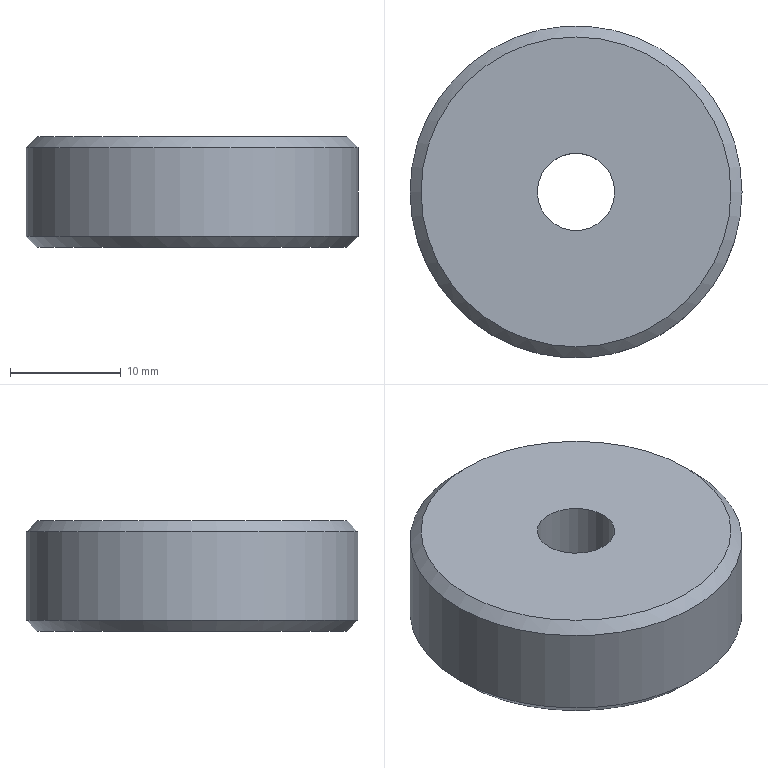Part | STEP file | solid 6 | 1 solid | 7 faces | box 30 x 30 x 10 mm | volume 6388 mm3 | cone 3 | plane 2 | cylinder 2 | commonest cylinder face diameters 7 x1 30 x1